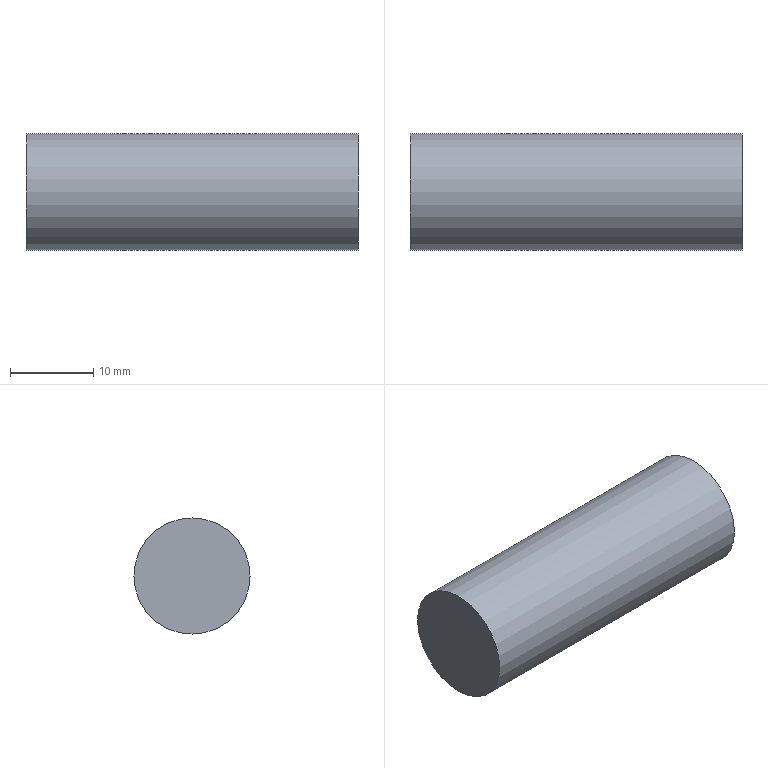Part | NX | features solid 2 | 1 solid | 3 faces | box 40 x 14 x 14 mm | volume 6158 mm3 | plane 2 | cylinder 1 | commonest cylinder face diameters 14 x1
STEP:
#1=CARTESIAN_POINT('',(-61.,145.3,103.));
#2=VERTEX_POINT('',#1);
#3=CARTESIAN_POINT('',(-61.,145.3,96.));
#4=DIRECTION('',(-1.,0.,0.));
#5=DIRECTION('',(0.,0.,1.));
#6=AXIS2_PLACEMENT_3D('',#3,#4,#5);
#7=CIRCLE('',#6,7.);
#8=EDGE_CURVE('',#2,#2,#7,.F.);
#9=ORIENTED_EDGE('',*,*,#8,.F.);
#10=EDGE_LOOP('',(#9));
#11=FACE_BOUND('',#10,.T.);
#12=CARTESIAN_POINT('',(-61.,145.3,96.));
#13=DIRECTION('',(-1.,0.,0.));
#14=DIRECTION('',(0.,0.,1.));
#15=AXIS2_PLACEMENT_3D('',#12,#13,#14);
#16=PLANE('',#15);
#17=ADVANCED_FACE('',(#11),#16,.T.);
#18=CARTESIAN_POINT('',(-21.,145.3,89.));
#19=VERTEX_POINT('',#18);
#20=CARTESIAN_POINT('',(-21.,145.3,96.));
#21=DIRECTION('',(1.,0.,0.));
#22=DIRECTION('',(0.,0.,-1.));
#23=AXIS2_PLACEMENT_3D('',#20,#21,#22);
#24=CIRCLE('',#23,7.);
#25=EDGE_CURVE('',#19,#19,#24,.F.);
#26=ORIENTED_EDGE('',*,*,#25,.F.);
#27=EDGE_LOOP('',(#26));
#28=FACE_BOUND('',#27,.T.);
#29=CARTESIAN_POINT('',(-21.,145.3,96.));
#30=DIRECTION('',(1.,0.,0.));
#31=DIRECTION('',(0.,0.,-1.));
#32=AXIS2_PLACEMENT_3D('',#29,#30,#31);
#33=PLANE('',#32);
#34=ADVANCED_FACE('',(#28),#33,.T.);
#35=ORIENTED_EDGE('',*,*,#8,.T.);
#36=EDGE_LOOP('',(#35));
#37=FACE_BOUND('',#36,.T.);
#38=ORIENTED_EDGE('',*,*,#25,.T.);
#39=EDGE_LOOP('',(#38));
#40=FACE_BOUND('',#39,.T.);
#41=CARTESIAN_POINT('',(-21.,145.3,96.));
#42=DIRECTION('',(-1.,0.,0.));
#43=DIRECTION('',(0.,0.,1.));
#44=AXIS2_PLACEMENT_3D('',#41,#42,#43);
#45=CYLINDRICAL_SURFACE('',#44,7.);
#46=ADVANCED_FACE('',(#37,#40),#45,.T.);
#47=CLOSED_SHELL('',(#17,#34,#46));
#48=MANIFOLD_SOLID_BREP('',#47);
#49=(LENGTH_UNIT()NAMED_UNIT(*)SI_UNIT(.MILLI.,.METRE.));
#50=UNCERTAINTY_MEASURE_WITH_UNIT(LENGTH_MEASURE(0.00001),#49,'','');
#51=(NAMED_UNIT(*)PLANE_ANGLE_UNIT()SI_UNIT($,.RADIAN.));
#52=(NAMED_UNIT(*)SI_UNIT($,.STERADIAN.)SOLID_ANGLE_UNIT());
#53=(GEOMETRIC_REPRESENTATION_CONTEXT(3)GLOBAL_UNCERTAINTY_ASSIGNED_CONTEXT((#50))GLOBAL_UNIT_ASSIGNED_CONTEXT((#49,#51,#52))REPRESENTATION_CONTEXT('',''));
#54=ADVANCED_BREP_SHAPE_REPRESENTATION('',(#48),#53);